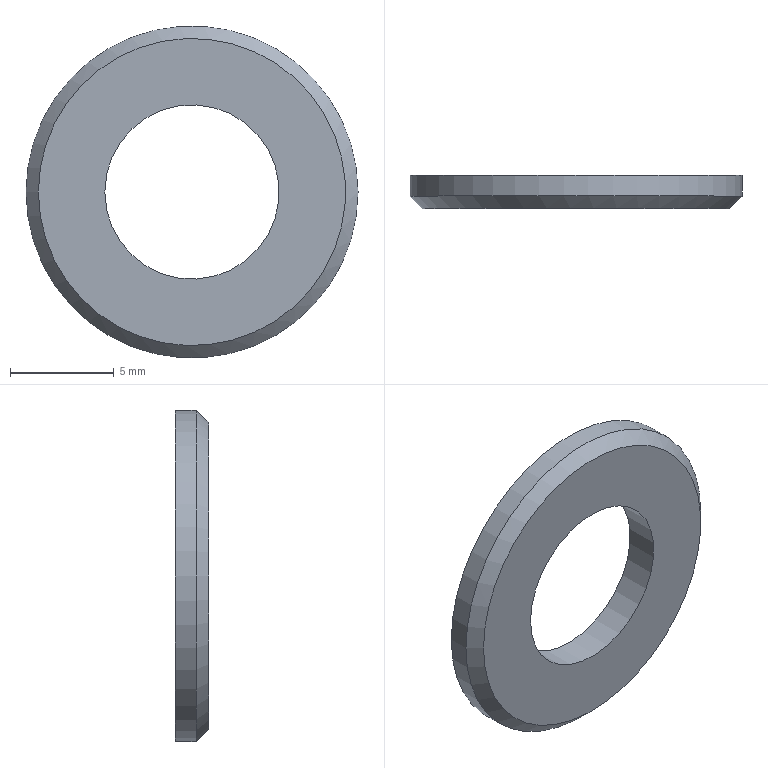Part | STEP file | Scheibe_DIN_125_1_B_8_4 | 1 solid | 5 faces | box 16 x 1.6 x 16 mm | volume 224.209 mm3 | plane 2 | cylinder 2 | cone 1 | commonest cylinder face diameters 8.4 x1 16 x1
STEP:
#1=CARTESIAN_POINT('',(0.,0.,0.));
#2=DIRECTION('',(0.,0.,1.));
#3=DIRECTION('',(1.,0.,0.));
#4=AXIS2_PLACEMENT_3D('',#1,#2,#3);
#5=CARTESIAN_POINT('',(-7.4,-1.6,0.));
#6=VERTEX_POINT('',#5);
#7=CARTESIAN_POINT('',(0.,-1.6,0.));
#8=DIRECTION('',(0.,1.,0.));
#9=DIRECTION('',(1.,0.,0.));
#10=AXIS2_PLACEMENT_3D('',#7,#8,#9);
#11=CIRCLE('',#10,7.4);
#12=CARTESIAN_POINT('',(0.,-1.,0.));
#13=DIRECTION('',(0.,1.,0.));
#14=DIRECTION('',(-1.,0.,0.));
#15=AXIS2_PLACEMENT_3D('',#12,#13,#14);
#16=CONICAL_SURFACE('',#15,8.,0.7854);
#17=CARTESIAN_POINT('',(-3.142,-0.6));
#18=DIRECTION('',(1.,0.));
#19=VECTOR('',#18,1.);
#20=LINE('',#17,#19);
#21=(GEOMETRIC_REPRESENTATION_CONTEXT(2)PARAMETRIC_REPRESENTATION_CONTEXT()REPRESENTATION_CONTEXT('',''));
#22=DEFINITIONAL_REPRESENTATION('',(#20),#21);
#23=PCURVE('',#16,#22);
#24=CARTESIAN_POINT('',(5.8,-1.6,0.));
#25=DIRECTION('',(0.,-1.,0.));
#26=DIRECTION('',(0.,0.,-1.));
#27=AXIS2_PLACEMENT_3D('',#24,#25,#26);
#28=PLANE('',#27);
#29=CARTESIAN_POINT('',(0.,1.6));
#30=CARTESIAN_POINT('',(12.817,1.6));
#31=CARTESIAN_POINT('',(6.409,-9.5));
#32=CARTESIAN_POINT('',(0.,-20.6));
#33=CARTESIAN_POINT('',(-6.409,-9.5));
#34=CARTESIAN_POINT('',(-12.817,1.6));
#35=CARTESIAN_POINT('',(0.,1.6));
#36=(BOUNDED_CURVE()B_SPLINE_CURVE(2,(#29,#30,#31,#32,#33,#34,#35),.UNSPECIFIED.,.T.,.F.)B_SPLINE_CURVE_WITH_KNOTS((1,2,2,2,2,1),(-2.094,0.,2.094,4.189,6.283,8.378),.UNSPECIFIED.)CURVE()GEOMETRIC_REPRESENTATION_ITEM()RATIONAL_B_SPLINE_CURVE((1.,0.5,1.,0.5,1.,0.5,1.))REPRESENTATION_ITEM(''));
#37=(GEOMETRIC_REPRESENTATION_CONTEXT(2)PARAMETRIC_REPRESENTATION_CONTEXT()REPRESENTATION_CONTEXT('',''));
#38=DEFINITIONAL_REPRESENTATION('',(#36),#37);
#39=PCURVE('',#28,#38);
#40=SURFACE_CURVE('',#11,(#23,#39),.PCURVE_S1.);
#41=EDGE_CURVE('',#6,#6,#40,.T.);
#42=ORIENTED_EDGE('',*,*,#41,.T.);
#43=CARTESIAN_POINT('',(-8.,-1.,0.));
#44=VERTEX_POINT('',#43);
#45=CARTESIAN_POINT('',(-7.4,-1.6,0.));
#46=CARTESIAN_POINT('',(-8.,-1.,0.));
#47=B_SPLINE_CURVE_WITH_KNOTS('',1,(#45,#46),.UNSPECIFIED.,.F.,.F.,(2,2),(-0.8485,0.),.PIECEWISE_BEZIER_KNOTS.);
#48=CARTESIAN_POINT('',(6.283,0.));
#49=DIRECTION('',(0.,1.));
#50=VECTOR('',#49,1.);
#51=LINE('',#48,#50);
#52=(GEOMETRIC_REPRESENTATION_CONTEXT(2)PARAMETRIC_REPRESENTATION_CONTEXT()REPRESENTATION_CONTEXT('',''));
#53=DEFINITIONAL_REPRESENTATION('',(#51),#52);
#54=PCURVE('',#16,#53);
#55=CARTESIAN_POINT('',(0.,0.));
#56=DIRECTION('',(0.,1.));
#57=VECTOR('',#56,1.);
#58=LINE('',#55,#57);
#59=(GEOMETRIC_REPRESENTATION_CONTEXT(2)PARAMETRIC_REPRESENTATION_CONTEXT()REPRESENTATION_CONTEXT('',''));
#60=DEFINITIONAL_REPRESENTATION('',(#58),#59);
#61=PCURVE('',#16,#60);
#62=SEAM_CURVE('',#47,(#54,#61),.PCURVE_S1.);
#63=EDGE_CURVE('',#6,#44,#62,.T.);
#64=ORIENTED_EDGE('',*,*,#63,.T.);
#65=CARTESIAN_POINT('',(0.,-1.,0.));
#66=DIRECTION('',(0.,1.,0.));
#67=DIRECTION('',(1.,0.,0.));
#68=AXIS2_PLACEMENT_3D('',#65,#66,#67);
#69=CIRCLE('',#68,8.);
#70=CARTESIAN_POINT('',(-3.142,0.));
#71=DIRECTION('',(1.,0.));
#72=VECTOR('',#71,1.);
#73=LINE('',#70,#72);
#74=(GEOMETRIC_REPRESENTATION_CONTEXT(2)PARAMETRIC_REPRESENTATION_CONTEXT()REPRESENTATION_CONTEXT('',''));
#75=DEFINITIONAL_REPRESENTATION('',(#73),#74);
#76=PCURVE('',#16,#75);
#77=CARTESIAN_POINT('',(0.,-0.5,0.));
#78=DIRECTION('',(0.,-1.,0.));
#79=DIRECTION('',(1.,0.,0.));
#80=AXIS2_PLACEMENT_3D('',#77,#78,#79);
#81=CYLINDRICAL_SURFACE('',#80,8.);
#82=CARTESIAN_POINT('',(12.566,0.5));
#83=DIRECTION('',(-1.,0.));
#84=VECTOR('',#83,1.);
#85=LINE('',#82,#84);
#86=(GEOMETRIC_REPRESENTATION_CONTEXT(2)PARAMETRIC_REPRESENTATION_CONTEXT()REPRESENTATION_CONTEXT('',''));
#87=DEFINITIONAL_REPRESENTATION('',(#85),#86);
#88=PCURVE('',#81,#87);
#89=SURFACE_CURVE('',#69,(#76,#88),.PCURVE_S1.);
#90=EDGE_CURVE('',#44,#44,#89,.T.);
#91=ORIENTED_EDGE('',*,*,#90,.F.);
#92=ORIENTED_EDGE('',*,*,#63,.F.);
#93=EDGE_LOOP('',(#42,#64,#91,#92));
#94=FACE_BOUND('',#93,.T.);
#95=ADVANCED_FACE('',(#94),#16,.T.);
#96=ORIENTED_EDGE('',*,*,#41,.F.);
#97=EDGE_LOOP('',(#96));
#98=FACE_BOUND('',#97,.T.);
#99=CARTESIAN_POINT('',(-4.2,-1.6,0.));
#100=VERTEX_POINT('',#99);
#101=CARTESIAN_POINT('',(0.,-1.6,0.));
#102=DIRECTION('',(0.,1.,0.));
#103=DIRECTION('',(1.,0.,0.));
#104=AXIS2_PLACEMENT_3D('',#101,#102,#103);
#105=CIRCLE('',#104,4.2);
#106=CARTESIAN_POINT('',(0.,-1.6));
#107=CARTESIAN_POINT('',(7.275,-1.6));
#108=CARTESIAN_POINT('',(3.637,-7.9));
#109=CARTESIAN_POINT('',(0.,-14.2));
#110=CARTESIAN_POINT('',(-3.637,-7.9));
#111=CARTESIAN_POINT('',(-7.275,-1.6));
#112=CARTESIAN_POINT('',(0.,-1.6));
#113=(BOUNDED_CURVE()B_SPLINE_CURVE(2,(#106,#107,#108,#109,#110,#111,#112),.UNSPECIFIED.,.T.,.F.)B_SPLINE_CURVE_WITH_KNOTS((1,2,2,2,2,1),(-2.094,0.,2.094,4.189,6.283,8.378),.UNSPECIFIED.)CURVE()GEOMETRIC_REPRESENTATION_ITEM()RATIONAL_B_SPLINE_CURVE((1.,0.5,1.,0.5,1.,0.5,1.))REPRESENTATION_ITEM(''));
#114=(GEOMETRIC_REPRESENTATION_CONTEXT(2)PARAMETRIC_REPRESENTATION_CONTEXT()REPRESENTATION_CONTEXT('',''));
#115=DEFINITIONAL_REPRESENTATION('',(#113),#114);
#116=PCURVE('',#28,#115);
#117=CARTESIAN_POINT('',(0.,-0.8,0.));
#118=DIRECTION('',(0.,-1.,0.));
#119=DIRECTION('',(1.,0.,0.));
#120=AXIS2_PLACEMENT_3D('',#117,#118,#119);
#121=CYLINDRICAL_SURFACE('',#120,4.2);
#122=CARTESIAN_POINT('',(12.566,0.8));
#123=DIRECTION('',(-1.,0.));
#124=VECTOR('',#123,1.);
#125=LINE('',#122,#124);
#126=(GEOMETRIC_REPRESENTATION_CONTEXT(2)PARAMETRIC_REPRESENTATION_CONTEXT()REPRESENTATION_CONTEXT('',''));
#127=DEFINITIONAL_REPRESENTATION('',(#125),#126);
#128=PCURVE('',#121,#127);
#129=SURFACE_CURVE('',#105,(#116,#128),.PCURVE_S1.);
#130=EDGE_CURVE('',#100,#100,#129,.T.);
#131=ORIENTED_EDGE('',*,*,#130,.T.);
#132=EDGE_LOOP('',(#131));
#133=FACE_BOUND('',#132,.T.);
#134=ADVANCED_FACE('',(#98,#133),#28,.T.);
#135=ORIENTED_EDGE('',*,*,#90,.T.);
#136=CARTESIAN_POINT('',(-8.,0.,0.));
#137=VERTEX_POINT('',#136);
#138=CARTESIAN_POINT('',(-8.,0.,0.));
#139=CARTESIAN_POINT('',(-8.,-1.,0.));
#140=B_SPLINE_CURVE_WITH_KNOTS('',1,(#138,#139),.UNSPECIFIED.,.F.,.F.,(2,2),(-0.5,0.5),.PIECEWISE_BEZIER_KNOTS.);
#141=CARTESIAN_POINT('',(3.142,0.));
#142=DIRECTION('',(0.,1.));
#143=VECTOR('',#142,1.);
#144=LINE('',#141,#143);
#145=(GEOMETRIC_REPRESENTATION_CONTEXT(2)PARAMETRIC_REPRESENTATION_CONTEXT()REPRESENTATION_CONTEXT('',''));
#146=DEFINITIONAL_REPRESENTATION('',(#144),#145);
#147=PCURVE('',#81,#146);
#148=CARTESIAN_POINT('',(9.425,0.));
#149=DIRECTION('',(0.,1.));
#150=VECTOR('',#149,1.);
#151=LINE('',#148,#150);
#152=(GEOMETRIC_REPRESENTATION_CONTEXT(2)PARAMETRIC_REPRESENTATION_CONTEXT()REPRESENTATION_CONTEXT('',''));
#153=DEFINITIONAL_REPRESENTATION('',(#151),#152);
#154=PCURVE('',#81,#153);
#155=SEAM_CURVE('',#140,(#147,#154),.PCURVE_S1.);
#156=EDGE_CURVE('',#137,#44,#155,.T.);
#157=ORIENTED_EDGE('',*,*,#156,.F.);
#158=CARTESIAN_POINT('',(0.,0.,0.));
#159=DIRECTION('',(0.,-1.,0.));
#160=DIRECTION('',(1.,0.,0.));
#161=AXIS2_PLACEMENT_3D('',#158,#159,#160);
#162=CIRCLE('',#161,8.);
#163=CARTESIAN_POINT('',(0.,-0.5));
#164=DIRECTION('',(1.,0.));
#165=VECTOR('',#164,1.);
#166=LINE('',#163,#165);
#167=(GEOMETRIC_REPRESENTATION_CONTEXT(2)PARAMETRIC_REPRESENTATION_CONTEXT()REPRESENTATION_CONTEXT('',''));
#168=DEFINITIONAL_REPRESENTATION('',(#166),#167);
#169=PCURVE('',#81,#168);
#170=CARTESIAN_POINT('',(6.1,0.,0.));
#171=DIRECTION('',(0.,-1.,0.));
#172=DIRECTION('',(0.,0.,-1.));
#173=AXIS2_PLACEMENT_3D('',#170,#171,#172);
#174=PLANE('',#173);
#175=CARTESIAN_POINT('',(0.,-6.1));
#176=DIRECTION('',(0.,1.));
#177=AXIS2_PLACEMENT_2D('',#175,#176);
#178=CIRCLE('',#177,8.);
#179=(GEOMETRIC_REPRESENTATION_CONTEXT(2)PARAMETRIC_REPRESENTATION_CONTEXT()REPRESENTATION_CONTEXT('',''));
#180=DEFINITIONAL_REPRESENTATION('',(#178),#179);
#181=PCURVE('',#174,#180);
#182=SURFACE_CURVE('',#162,(#169,#181),.PCURVE_S1.);
#183=EDGE_CURVE('',#137,#137,#182,.T.);
#184=ORIENTED_EDGE('',*,*,#183,.T.);
#185=ORIENTED_EDGE('',*,*,#156,.T.);
#186=EDGE_LOOP('',(#135,#157,#184,#185));
#187=FACE_BOUND('',#186,.T.);
#188=ADVANCED_FACE('',(#187),#81,.T.);
#189=CARTESIAN_POINT('',(-4.2,0.000000001,0.));
#190=VERTEX_POINT('',#189);
#191=CARTESIAN_POINT('',(0.,0.,0.));
#192=DIRECTION('',(0.,1.,0.));
#193=DIRECTION('',(1.,0.,0.));
#194=AXIS2_PLACEMENT_3D('',#191,#192,#193);
#195=CIRCLE('',#194,4.2);
#196=CARTESIAN_POINT('',(12.566,-0.8));
#197=DIRECTION('',(-1.,0.));
#198=VECTOR('',#197,1.);
#199=LINE('',#196,#198);
#200=(GEOMETRIC_REPRESENTATION_CONTEXT(2)PARAMETRIC_REPRESENTATION_CONTEXT()REPRESENTATION_CONTEXT('',''));
#201=DEFINITIONAL_REPRESENTATION('',(#199),#200);
#202=PCURVE('',#121,#201);
#203=CARTESIAN_POINT('',(0.,-1.9));
#204=CARTESIAN_POINT('',(7.275,-1.9));
#205=CARTESIAN_POINT('',(3.637,-8.2));
#206=CARTESIAN_POINT('',(0.,-14.5));
#207=CARTESIAN_POINT('',(-3.637,-8.2));
#208=CARTESIAN_POINT('',(-7.275,-1.9));
#209=CARTESIAN_POINT('',(0.,-1.9));
#210=(BOUNDED_CURVE()B_SPLINE_CURVE(2,(#203,#204,#205,#206,#207,#208,#209),.UNSPECIFIED.,.T.,.F.)B_SPLINE_CURVE_WITH_KNOTS((1,2,2,2,2,1),(-2.094,0.,2.094,4.189,6.283,8.378),.UNSPECIFIED.)CURVE()GEOMETRIC_REPRESENTATION_ITEM()RATIONAL_B_SPLINE_CURVE((1.,0.5,1.,0.5,1.,0.5,1.))REPRESENTATION_ITEM(''));
#211=(GEOMETRIC_REPRESENTATION_CONTEXT(2)PARAMETRIC_REPRESENTATION_CONTEXT()REPRESENTATION_CONTEXT('',''));
#212=DEFINITIONAL_REPRESENTATION('',(#210),#211);
#213=PCURVE('',#174,#212);
#214=SURFACE_CURVE('',#195,(#202,#213),.PCURVE_S1.);
#215=EDGE_CURVE('',#190,#190,#214,.T.);
#216=ORIENTED_EDGE('',*,*,#215,.F.);
#217=CARTESIAN_POINT('',(-4.2,0.000000001,0.));
#218=CARTESIAN_POINT('',(-4.2,-1.6,0.));
#219=B_SPLINE_CURVE_WITH_KNOTS('',1,(#217,#218),.UNSPECIFIED.,.F.,.F.,(2,2),(-0.8,0.8),.PIECEWISE_BEZIER_KNOTS.);
#220=CARTESIAN_POINT('',(9.425,0.));
#221=DIRECTION('',(0.,1.));
#222=VECTOR('',#221,1.);
#223=LINE('',#220,#222);
#224=(GEOMETRIC_REPRESENTATION_CONTEXT(2)PARAMETRIC_REPRESENTATION_CONTEXT()REPRESENTATION_CONTEXT('',''));
#225=DEFINITIONAL_REPRESENTATION('',(#223),#224);
#226=PCURVE('',#121,#225);
#227=CARTESIAN_POINT('',(3.142,0.));
#228=DIRECTION('',(0.,1.));
#229=VECTOR('',#228,1.);
#230=LINE('',#227,#229);
#231=(GEOMETRIC_REPRESENTATION_CONTEXT(2)PARAMETRIC_REPRESENTATION_CONTEXT()REPRESENTATION_CONTEXT('',''));
#232=DEFINITIONAL_REPRESENTATION('',(#230),#231);
#233=PCURVE('',#121,#232);
#234=SEAM_CURVE('',#219,(#226,#233),.PCURVE_S1.);
#235=EDGE_CURVE('',#190,#100,#234,.T.);
#236=ORIENTED_EDGE('',*,*,#235,.T.);
#237=ORIENTED_EDGE('',*,*,#130,.T.);
#238=ORIENTED_EDGE('',*,*,#235,.F.);
#239=EDGE_LOOP('',(#216,#236,#237,#238));
#240=FACE_BOUND('',#239,.F.);
#241=ADVANCED_FACE('',(#240),#121,.F.);
#242=ORIENTED_EDGE('',*,*,#183,.F.);
#243=EDGE_LOOP('',(#242));
#244=FACE_BOUND('',#243,.T.);
#245=ORIENTED_EDGE('',*,*,#215,.F.);
#246=EDGE_LOOP('',(#245));
#247=FACE_BOUND('',#246,.T.);
#248=ADVANCED_FACE('',(#244,#247),#174,.F.);
#249=CLOSED_SHELL('',(#95,#134,#188,#241,#248));
#250=MANIFOLD_SOLID_BREP('',#249);
#251=(LENGTH_UNIT()NAMED_UNIT(*)SI_UNIT(.MILLI.,.METRE.));
#252=UNCERTAINTY_MEASURE_WITH_UNIT(LENGTH_MEASURE(0.00001),#251,'','');
#253=(NAMED_UNIT(*)PLANE_ANGLE_UNIT()SI_UNIT($,.RADIAN.));
#254=(NAMED_UNIT(*)SI_UNIT($,.STERADIAN.)SOLID_ANGLE_UNIT());
#255=(GEOMETRIC_REPRESENTATION_CONTEXT(3)GLOBAL_UNCERTAINTY_ASSIGNED_CONTEXT((#252))GLOBAL_UNIT_ASSIGNED_CONTEXT((#251,#253,#254))REPRESENTATION_CONTEXT('',''));
#256=ADVANCED_BREP_SHAPE_REPRESENTATION('',(#4,#250),#255);